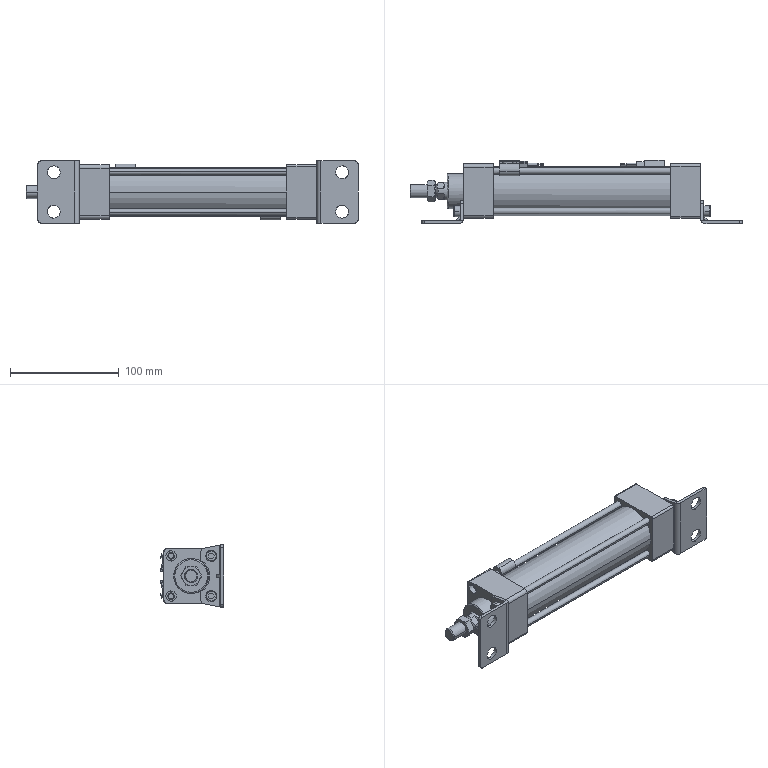Part | SolidWorks | features AEMSimFeature 1 | 13 solids | 538 faces | box 305 x 58.518 x 57 mm | volume 304092 mm3 | plane 242 | cylinder 200 | cone 86 | torus 10 | commonest cylinder face diameters 6 x20 4.917 x16 9.5 x16 4 x14 5 x12 12 x12